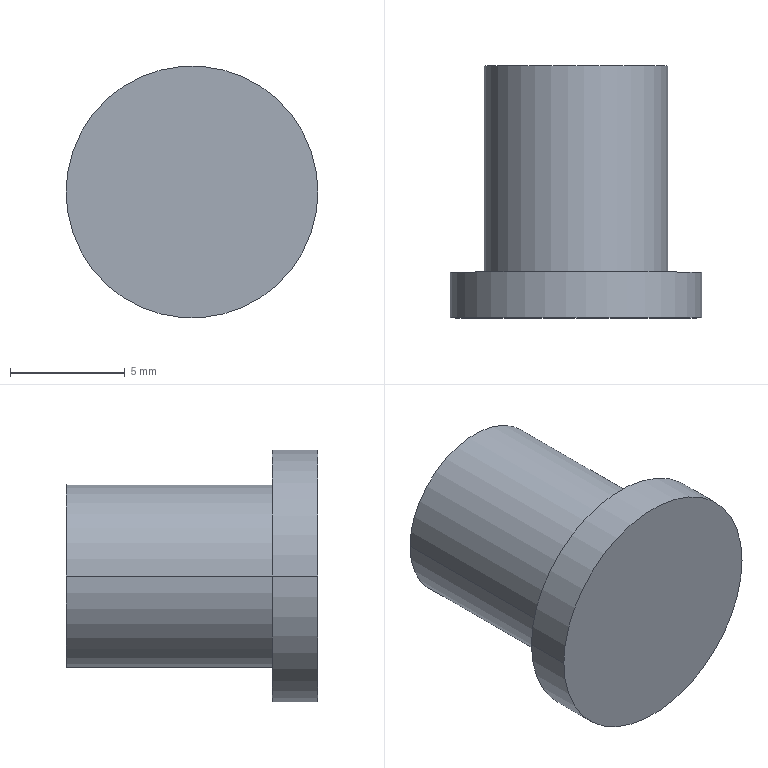Part | SolidWorks | features BaseBody 1 | 1 solid | 7 faces | box 11 x 11 x 11 mm | volume 642.456 mm3 | cylinder 4 | plane 3 | commonest cylinder face diameters 8 x2 11 x2
STEP:
#1=CARTESIAN_POINT('',(4.,11.,0.));
#2=VERTEX_POINT('',#1);
#3=CARTESIAN_POINT('',(-4.,11.,0.));
#4=VERTEX_POINT('',#3);
#5=CARTESIAN_POINT('',(0.,11.,0.));
#6=DIRECTION('',(0.,-1.,0.));
#7=DIRECTION('',(1.,0.,0.));
#8=AXIS2_PLACEMENT_3D('',#5,#6,#7);
#9=CIRCLE('',#8,4.);
#10=EDGE_CURVE('',#2,#4,#9,.T.);
#11=ORIENTED_EDGE('',*,*,#10,.T.);
#12=CARTESIAN_POINT('',(-4.,2.,0.));
#13=VERTEX_POINT('',#12);
#14=CARTESIAN_POINT('',(-4.,-326.901,0.));
#15=DIRECTION('',(0.,-1.,0.));
#16=VECTOR('',#15,1000.);
#17=LINE('',#14,#16);
#18=EDGE_CURVE('',#4,#13,#17,.T.);
#19=ORIENTED_EDGE('',*,*,#18,.T.);
#20=CARTESIAN_POINT('',(4.,2.,0.));
#21=VERTEX_POINT('',#20);
#22=CARTESIAN_POINT('',(0.,2.,0.));
#23=DIRECTION('',(0.,1.,0.));
#24=DIRECTION('',(1.,0.,0.));
#25=AXIS2_PLACEMENT_3D('',#22,#23,#24);
#26=CIRCLE('',#25,4.);
#27=EDGE_CURVE('',#13,#21,#26,.T.);
#28=ORIENTED_EDGE('',*,*,#27,.T.);
#29=CARTESIAN_POINT('',(4.,-326.901,0.));
#30=DIRECTION('',(0.,-1.,0.));
#31=VECTOR('',#30,1000.);
#32=LINE('',#29,#31);
#33=EDGE_CURVE('',#2,#21,#32,.T.);
#34=ORIENTED_EDGE('',*,*,#33,.F.);
#35=EDGE_LOOP('',(#11,#19,#28,#34));
#36=FACE_OUTER_BOUND('',#35,.T.);
#37=CARTESIAN_POINT('',(0.,-326.901,0.));
#38=DIRECTION('',(0.,-1.,0.));
#39=DIRECTION('',(1.,0.,0.));
#40=AXIS2_PLACEMENT_3D('',#37,#38,#39);
#41=CYLINDRICAL_SURFACE('',#40,4.);
#42=ADVANCED_FACE('',(#36),#41,.T.);
#43=CARTESIAN_POINT('',(-5.5,2.,0.));
#44=VERTEX_POINT('',#43);
#45=CARTESIAN_POINT('',(5.5,2.,0.));
#46=VERTEX_POINT('',#45);
#47=CARTESIAN_POINT('',(0.,2.,0.));
#48=DIRECTION('',(0.,1.,0.));
#49=DIRECTION('',(1.,0.,0.));
#50=AXIS2_PLACEMENT_3D('',#47,#48,#49);
#51=CIRCLE('',#50,5.5);
#52=EDGE_CURVE('',#44,#46,#51,.T.);
#53=ORIENTED_EDGE('',*,*,#52,.F.);
#54=CARTESIAN_POINT('',(-5.5,0.,0.));
#55=VERTEX_POINT('',#54);
#56=CARTESIAN_POINT('',(-5.5,-326.901,0.));
#57=DIRECTION('',(0.,-1.,0.));
#58=VECTOR('',#57,1000.);
#59=LINE('',#56,#58);
#60=EDGE_CURVE('',#44,#55,#59,.T.);
#61=ORIENTED_EDGE('',*,*,#60,.T.);
#62=CARTESIAN_POINT('',(5.5,0.,0.));
#63=VERTEX_POINT('',#62);
#64=CARTESIAN_POINT('',(0.,0.,0.));
#65=DIRECTION('',(0.,1.,0.));
#66=DIRECTION('',(1.,0.,0.));
#67=AXIS2_PLACEMENT_3D('',#64,#65,#66);
#68=CIRCLE('',#67,5.5);
#69=EDGE_CURVE('',#55,#63,#68,.T.);
#70=ORIENTED_EDGE('',*,*,#69,.T.);
#71=CARTESIAN_POINT('',(5.5,-326.901,0.));
#72=DIRECTION('',(0.,-1.,0.));
#73=VECTOR('',#72,1000.);
#74=LINE('',#71,#73);
#75=EDGE_CURVE('',#46,#63,#74,.T.);
#76=ORIENTED_EDGE('',*,*,#75,.F.);
#77=EDGE_LOOP('',(#53,#61,#70,#76));
#78=FACE_OUTER_BOUND('',#77,.T.);
#79=CARTESIAN_POINT('',(0.,-326.901,0.));
#80=DIRECTION('',(0.,-1.,0.));
#81=DIRECTION('',(1.,0.,0.));
#82=AXIS2_PLACEMENT_3D('',#79,#80,#81);
#83=CYLINDRICAL_SURFACE('',#82,5.5);
#84=ADVANCED_FACE('',(#78),#83,.T.);
#85=ORIENTED_EDGE('',*,*,#18,.F.);
#86=CARTESIAN_POINT('',(0.,11.,0.));
#87=DIRECTION('',(0.,-1.,0.));
#88=DIRECTION('',(1.,0.,0.));
#89=AXIS2_PLACEMENT_3D('',#86,#87,#88);
#90=CIRCLE('',#89,4.);
#91=EDGE_CURVE('',#4,#2,#90,.T.);
#92=ORIENTED_EDGE('',*,*,#91,.T.);
#93=ORIENTED_EDGE('',*,*,#33,.T.);
#94=CARTESIAN_POINT('',(0.,2.,0.));
#95=DIRECTION('',(0.,1.,0.));
#96=DIRECTION('',(1.,0.,0.));
#97=AXIS2_PLACEMENT_3D('',#94,#95,#96);
#98=CIRCLE('',#97,4.);
#99=EDGE_CURVE('',#21,#13,#98,.T.);
#100=ORIENTED_EDGE('',*,*,#99,.T.);
#101=EDGE_LOOP('',(#85,#92,#93,#100));
#102=FACE_OUTER_BOUND('',#101,.T.);
#103=CARTESIAN_POINT('',(0.,-326.901,0.));
#104=DIRECTION('',(0.,-1.,0.));
#105=DIRECTION('',(1.,0.,0.));
#106=AXIS2_PLACEMENT_3D('',#103,#104,#105);
#107=CYLINDRICAL_SURFACE('',#106,4.);
#108=ADVANCED_FACE('',(#102),#107,.T.);
#109=ORIENTED_EDGE('',*,*,#99,.F.);
#110=ORIENTED_EDGE('',*,*,#27,.F.);
#111=EDGE_LOOP('',(#109,#110));
#112=FACE_BOUND('',#111,.T.);
#113=CARTESIAN_POINT('',(0.,2.,0.));
#114=DIRECTION('',(0.,1.,0.));
#115=DIRECTION('',(1.,0.,0.));
#116=AXIS2_PLACEMENT_3D('',#113,#114,#115);
#117=CIRCLE('',#116,5.5);
#118=EDGE_CURVE('',#46,#44,#117,.T.);
#119=ORIENTED_EDGE('',*,*,#118,.T.);
#120=ORIENTED_EDGE('',*,*,#52,.T.);
#121=EDGE_LOOP('',(#119,#120));
#122=FACE_OUTER_BOUND('',#121,.T.);
#123=CARTESIAN_POINT('',(4.,2.,0.));
#124=DIRECTION('',(0.,1.,0.));
#125=DIRECTION('',(-1.,0.,0.));
#126=AXIS2_PLACEMENT_3D('',#123,#124,#125);
#127=PLANE('',#126);
#128=ADVANCED_FACE('',(#112,#122),#127,.T.);
#129=ORIENTED_EDGE('',*,*,#10,.F.);
#130=ORIENTED_EDGE('',*,*,#91,.F.);
#131=EDGE_LOOP('',(#129,#130));
#132=FACE_OUTER_BOUND('',#131,.T.);
#133=CARTESIAN_POINT('',(0.,11.,0.));
#134=DIRECTION('',(0.,1.,0.));
#135=DIRECTION('',(-1.,0.,0.));
#136=AXIS2_PLACEMENT_3D('',#133,#134,#135);
#137=PLANE('',#136);
#138=ADVANCED_FACE('',(#132),#137,.T.);
#139=ORIENTED_EDGE('',*,*,#60,.F.);
#140=ORIENTED_EDGE('',*,*,#118,.F.);
#141=ORIENTED_EDGE('',*,*,#75,.T.);
#142=CARTESIAN_POINT('',(0.,0.,0.));
#143=DIRECTION('',(0.,1.,0.));
#144=DIRECTION('',(1.,0.,0.));
#145=AXIS2_PLACEMENT_3D('',#142,#143,#144);
#146=CIRCLE('',#145,5.5);
#147=EDGE_CURVE('',#63,#55,#146,.T.);
#148=ORIENTED_EDGE('',*,*,#147,.T.);
#149=EDGE_LOOP('',(#139,#140,#141,#148));
#150=FACE_OUTER_BOUND('',#149,.T.);
#151=CARTESIAN_POINT('',(0.,-326.901,0.));
#152=DIRECTION('',(0.,-1.,0.));
#153=DIRECTION('',(1.,0.,0.));
#154=AXIS2_PLACEMENT_3D('',#151,#152,#153);
#155=CYLINDRICAL_SURFACE('',#154,5.5);
#156=ADVANCED_FACE('',(#150),#155,.T.);
#157=ORIENTED_EDGE('',*,*,#147,.F.);
#158=ORIENTED_EDGE('',*,*,#69,.F.);
#159=EDGE_LOOP('',(#157,#158));
#160=FACE_OUTER_BOUND('',#159,.T.);
#161=CARTESIAN_POINT('',(5.5,0.,0.));
#162=DIRECTION('',(0.,-1.,0.));
#163=DIRECTION('',(1.,0.,0.));
#164=AXIS2_PLACEMENT_3D('',#161,#162,#163);
#165=PLANE('',#164);
#166=ADVANCED_FACE('',(#160),#165,.T.);
#167=CLOSED_SHELL('',(#42,#84,#108,#128,#138,#156,#166));
#168=MANIFOLD_SOLID_BREP('',#167);
#169=CARTESIAN_POINT('',(0.,0.,0.));
#170=DIRECTION('',(0.,0.,1.));
#171=DIRECTION('',(1.,0.,0.));
#172=AXIS2_PLACEMENT_3D('',#169,#170,#171);
#173=(LENGTH_UNIT()NAMED_UNIT(*)SI_UNIT(.MILLI.,.METRE.));
#174=UNCERTAINTY_MEASURE_WITH_UNIT(LENGTH_MEASURE(0.00001),#173,'','');
#175=(NAMED_UNIT(*)PLANE_ANGLE_UNIT()SI_UNIT($,.RADIAN.));
#176=(NAMED_UNIT(*)SI_UNIT($,.STERADIAN.)SOLID_ANGLE_UNIT());
#177=(GEOMETRIC_REPRESENTATION_CONTEXT(3)GLOBAL_UNCERTAINTY_ASSIGNED_CONTEXT((#174))GLOBAL_UNIT_ASSIGNED_CONTEXT((#173,#175,#176))REPRESENTATION_CONTEXT('',''));
#178=ADVANCED_BREP_SHAPE_REPRESENTATION('',(#168,#172),#177);